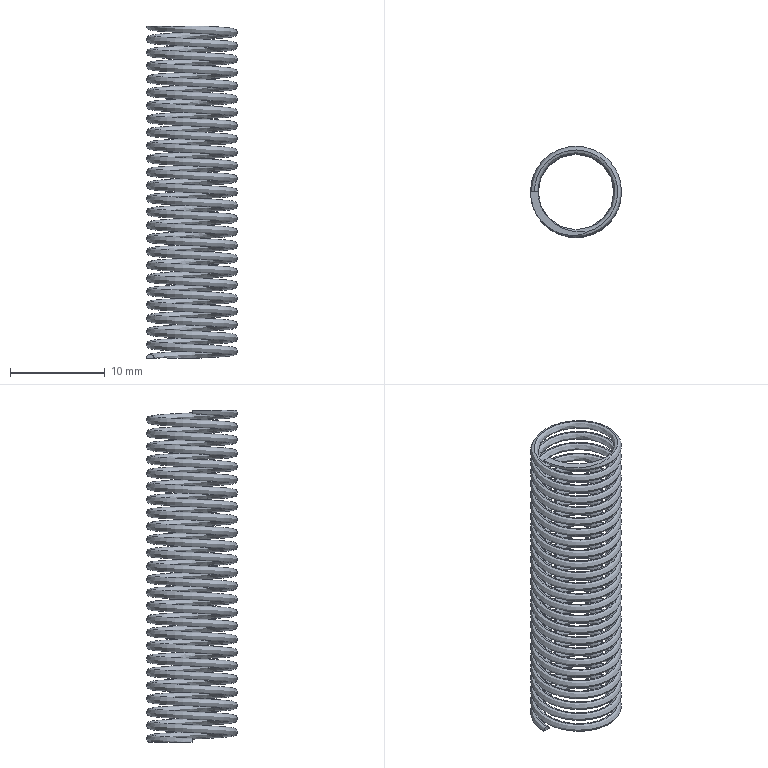Part | STEP file | spring 2 | 1 solid | 6 faces | box 9.6 x 9.6 x 35 mm | volume 344.84 mm3 | plane 4 | spline 2